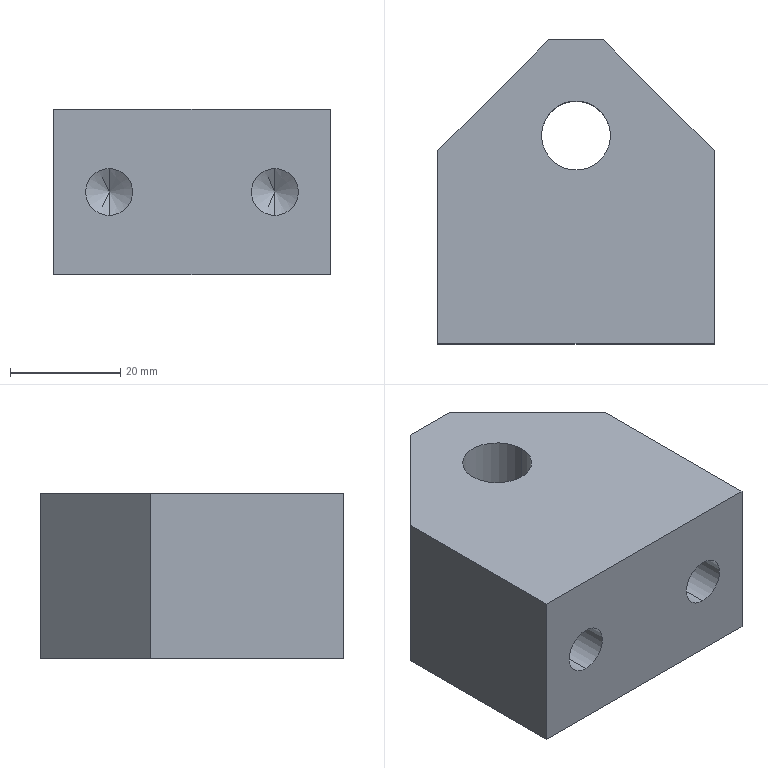Part | SolidWorks | features Chamfer 1, Extrusion 1, HoleWzd 1, ICE 1 | 1 solid | 18 faces | box 50 x 55 x 30 mm | volume 63941 mm3 | plane 8 | cylinder 6 | cone 4 | commonest cylinder face diameters 8.5 x4 12.5 x2
STEP:
#1=CARTESIAN_POINT('',(-6.25,10.2,0.));
#2=VERTEX_POINT('',#1);
#3=CARTESIAN_POINT('',(6.25,10.2,0.));
#4=VERTEX_POINT('',#3);
#5=CARTESIAN_POINT('',(0.,10.2,0.));
#6=DIRECTION('',(0.,0.,1.));
#7=DIRECTION('',(1.,0.,0.));
#8=AXIS2_PLACEMENT_3D('',#5,#6,#7);
#9=CIRCLE('',#8,6.25);
#10=EDGE_CURVE('',#2,#4,#9,.T.);
#11=ORIENTED_EDGE('',*,*,#10,.F.);
#12=CARTESIAN_POINT('',(-6.25,10.2,30.));
#13=VERTEX_POINT('',#12);
#14=CARTESIAN_POINT('',(-6.25,10.2,0.));
#15=DIRECTION('',(0.,0.,1.));
#16=VECTOR('',#15,1000.);
#17=LINE('',#14,#16);
#18=EDGE_CURVE('',#2,#13,#17,.T.);
#19=ORIENTED_EDGE('',*,*,#18,.T.);
#20=CARTESIAN_POINT('',(6.25,10.2,30.));
#21=VERTEX_POINT('',#20);
#22=CARTESIAN_POINT('',(0.,10.2,30.));
#23=DIRECTION('',(0.,0.,1.));
#24=DIRECTION('',(1.,0.,0.));
#25=AXIS2_PLACEMENT_3D('',#22,#23,#24);
#26=CIRCLE('',#25,6.25);
#27=EDGE_CURVE('',#13,#21,#26,.T.);
#28=ORIENTED_EDGE('',*,*,#27,.T.);
#29=CARTESIAN_POINT('',(6.25,10.2,0.));
#30=DIRECTION('',(0.,0.,1.));
#31=VECTOR('',#30,1000.);
#32=LINE('',#29,#31);
#33=EDGE_CURVE('',#4,#21,#32,.T.);
#34=ORIENTED_EDGE('',*,*,#33,.F.);
#35=EDGE_LOOP('',(#11,#19,#28,#34));
#36=FACE_OUTER_BOUND('',#35,.T.);
#37=CARTESIAN_POINT('',(0.,10.2,0.));
#38=DIRECTION('',(0.,0.,1.));
#39=DIRECTION('',(1.,0.,0.));
#40=AXIS2_PLACEMENT_3D('',#37,#38,#39);
#41=CYLINDRICAL_SURFACE('',#40,6.25);
#42=ADVANCED_FACE('',(#36),#41,.F.);
#43=CARTESIAN_POINT('',(-15.,-3.,19.25));
#44=VERTEX_POINT('',#43);
#45=CARTESIAN_POINT('',(-15.,-3.,10.75));
#46=VERTEX_POINT('',#45);
#47=CARTESIAN_POINT('',(-15.,-3.,15.));
#48=DIRECTION('',(0.,-1.,0.));
#49=DIRECTION('',(0.,0.,-1.));
#50=AXIS2_PLACEMENT_3D('',#47,#48,#49);
#51=CIRCLE('',#50,4.25);
#52=EDGE_CURVE('',#44,#46,#51,.T.);
#53=ORIENTED_EDGE('',*,*,#52,.F.);
#54=CARTESIAN_POINT('',(-15.,-27.5,19.25));
#55=VERTEX_POINT('',#54);
#56=CARTESIAN_POINT('',(-15.,-27.5,19.25));
#57=DIRECTION('',(0.,-1.,0.));
#58=VECTOR('',#57,1000.);
#59=LINE('',#56,#58);
#60=EDGE_CURVE('',#44,#55,#59,.T.);
#61=ORIENTED_EDGE('',*,*,#60,.T.);
#62=CARTESIAN_POINT('',(-15.,-27.5,10.75));
#63=VERTEX_POINT('',#62);
#64=CARTESIAN_POINT('',(-15.,-27.5,15.));
#65=DIRECTION('',(0.,-1.,0.));
#66=DIRECTION('',(0.,0.,-1.));
#67=AXIS2_PLACEMENT_3D('',#64,#65,#66);
#68=CIRCLE('',#67,4.25);
#69=EDGE_CURVE('',#55,#63,#68,.T.);
#70=ORIENTED_EDGE('',*,*,#69,.T.);
#71=CARTESIAN_POINT('',(-15.,-27.5,10.75));
#72=DIRECTION('',(0.,-1.,0.));
#73=VECTOR('',#72,1000.);
#74=LINE('',#71,#73);
#75=EDGE_CURVE('',#46,#63,#74,.T.);
#76=ORIENTED_EDGE('',*,*,#75,.F.);
#77=EDGE_LOOP('',(#53,#61,#70,#76));
#78=FACE_OUTER_BOUND('',#77,.T.);
#79=CARTESIAN_POINT('',(-15.,-27.5,15.));
#80=DIRECTION('',(0.,-1.,0.));
#81=DIRECTION('',(0.,0.,-1.));
#82=AXIS2_PLACEMENT_3D('',#79,#80,#81);
#83=CYLINDRICAL_SURFACE('',#82,4.25);
#84=ADVANCED_FACE('',(#78),#83,.F.);
#85=CARTESIAN_POINT('',(-15.,-0.4463,15.));
#86=VERTEX_POINT('',#85);
#87=CARTESIAN_POINT('',(-15.,-3.,10.75));
#88=DIRECTION('',(0.,-0.515,-0.8572));
#89=VECTOR('',#88,1000.);
#90=LINE('',#87,#89);
#91=EDGE_CURVE('',#86,#46,#90,.T.);
#92=ORIENTED_EDGE('',*,*,#91,.F.);
#93=CARTESIAN_POINT('',(-15.,-3.,19.25));
#94=DIRECTION('',(0.,-0.515,0.8572));
#95=VECTOR('',#94,1000.);
#96=LINE('',#93,#95);
#97=EDGE_CURVE('',#86,#44,#96,.T.);
#98=ORIENTED_EDGE('',*,*,#97,.T.);
#99=ORIENTED_EDGE('',*,*,#52,.T.);
#100=EDGE_LOOP('',(#92,#98,#99));
#101=FACE_OUTER_BOUND('',#100,.T.);
#102=CARTESIAN_POINT('',(-15.,-3.,15.));
#103=DIRECTION('',(0.,-1.,0.));
#104=DIRECTION('',(0.,0.,-1.));
#105=AXIS2_PLACEMENT_3D('',#102,#103,#104);
#106=CONICAL_SURFACE('',#105,4.25,1.03);
#107=ADVANCED_FACE('',(#101),#106,.F.);
#108=CARTESIAN_POINT('',(15.,-3.,19.25));
#109=VERTEX_POINT('',#108);
#110=CARTESIAN_POINT('',(15.,-3.,10.75));
#111=VERTEX_POINT('',#110);
#112=CARTESIAN_POINT('',(15.,-3.,15.));
#113=DIRECTION('',(0.,-1.,0.));
#114=DIRECTION('',(0.,0.,-1.));
#115=AXIS2_PLACEMENT_3D('',#112,#113,#114);
#116=CIRCLE('',#115,4.25);
#117=EDGE_CURVE('',#109,#111,#116,.T.);
#118=ORIENTED_EDGE('',*,*,#117,.F.);
#119=CARTESIAN_POINT('',(15.,-27.5,19.25));
#120=VERTEX_POINT('',#119);
#121=CARTESIAN_POINT('',(15.,-27.5,19.25));
#122=DIRECTION('',(0.,-1.,0.));
#123=VECTOR('',#122,1000.);
#124=LINE('',#121,#123);
#125=EDGE_CURVE('',#109,#120,#124,.T.);
#126=ORIENTED_EDGE('',*,*,#125,.T.);
#127=CARTESIAN_POINT('',(15.,-27.5,10.75));
#128=VERTEX_POINT('',#127);
#129=CARTESIAN_POINT('',(15.,-27.5,15.));
#130=DIRECTION('',(0.,-1.,0.));
#131=DIRECTION('',(0.,0.,-1.));
#132=AXIS2_PLACEMENT_3D('',#129,#130,#131);
#133=CIRCLE('',#132,4.25);
#134=EDGE_CURVE('',#120,#128,#133,.T.);
#135=ORIENTED_EDGE('',*,*,#134,.T.);
#136=CARTESIAN_POINT('',(15.,-27.5,10.75));
#137=DIRECTION('',(0.,-1.,0.));
#138=VECTOR('',#137,1000.);
#139=LINE('',#136,#138);
#140=EDGE_CURVE('',#111,#128,#139,.T.);
#141=ORIENTED_EDGE('',*,*,#140,.F.);
#142=EDGE_LOOP('',(#118,#126,#135,#141));
#143=FACE_OUTER_BOUND('',#142,.T.);
#144=CARTESIAN_POINT('',(15.,-27.5,15.));
#145=DIRECTION('',(0.,-1.,0.));
#146=DIRECTION('',(0.,0.,-1.));
#147=AXIS2_PLACEMENT_3D('',#144,#145,#146);
#148=CYLINDRICAL_SURFACE('',#147,4.25);
#149=ADVANCED_FACE('',(#143),#148,.F.);
#150=CARTESIAN_POINT('',(15.,-0.4463,15.));
#151=VERTEX_POINT('',#150);
#152=CARTESIAN_POINT('',(15.,-3.,10.75));
#153=DIRECTION('',(0.,-0.515,-0.8572));
#154=VECTOR('',#153,1000.);
#155=LINE('',#152,#154);
#156=EDGE_CURVE('',#151,#111,#155,.T.);
#157=ORIENTED_EDGE('',*,*,#156,.F.);
#158=CARTESIAN_POINT('',(15.,-3.,19.25));
#159=DIRECTION('',(0.,-0.515,0.8572));
#160=VECTOR('',#159,1000.);
#161=LINE('',#158,#160);
#162=EDGE_CURVE('',#151,#109,#161,.T.);
#163=ORIENTED_EDGE('',*,*,#162,.T.);
#164=ORIENTED_EDGE('',*,*,#117,.T.);
#165=EDGE_LOOP('',(#157,#163,#164));
#166=FACE_OUTER_BOUND('',#165,.T.);
#167=CARTESIAN_POINT('',(15.,-3.,15.));
#168=DIRECTION('',(0.,-1.,0.));
#169=DIRECTION('',(0.,0.,-1.));
#170=AXIS2_PLACEMENT_3D('',#167,#168,#169);
#171=CONICAL_SURFACE('',#170,4.25,1.03);
#172=ADVANCED_FACE('',(#166),#171,.F.);
#173=CARTESIAN_POINT('',(25.,-27.5,0.));
#174=VERTEX_POINT('',#173);
#175=CARTESIAN_POINT('',(25.,7.5,0.));
#176=VERTEX_POINT('',#175);
#177=CARTESIAN_POINT('',(25.,27.5,0.));
#178=DIRECTION('',(0.,1.,0.));
#179=VECTOR('',#178,1000.);
#180=LINE('',#177,#179);
#181=EDGE_CURVE('',#174,#176,#180,.T.);
#182=ORIENTED_EDGE('',*,*,#181,.T.);
#183=CARTESIAN_POINT('',(25.,7.5,30.));
#184=VERTEX_POINT('',#183);
#185=CARTESIAN_POINT('',(25.,7.5,30.));
#186=DIRECTION('',(0.,0.,1.));
#187=VECTOR('',#186,1000.);
#188=LINE('',#185,#187);
#189=EDGE_CURVE('',#176,#184,#188,.T.);
#190=ORIENTED_EDGE('',*,*,#189,.T.);
#191=CARTESIAN_POINT('',(25.,-27.5,30.));
#192=VERTEX_POINT('',#191);
#193=CARTESIAN_POINT('',(25.,27.5,30.));
#194=DIRECTION('',(0.,1.,0.));
#195=VECTOR('',#194,1000.);
#196=LINE('',#193,#195);
#197=EDGE_CURVE('',#192,#184,#196,.T.);
#198=ORIENTED_EDGE('',*,*,#197,.F.);
#199=CARTESIAN_POINT('',(25.,-27.5,30.));
#200=DIRECTION('',(0.,0.,-1.));
#201=VECTOR('',#200,1000.);
#202=LINE('',#199,#201);
#203=EDGE_CURVE('',#192,#174,#202,.T.);
#204=ORIENTED_EDGE('',*,*,#203,.T.);
#205=EDGE_LOOP('',(#182,#190,#198,#204));
#206=FACE_OUTER_BOUND('',#205,.T.);
#207=CARTESIAN_POINT('',(25.,27.5,30.));
#208=DIRECTION('',(-1.,0.,0.));
#209=DIRECTION('',(0.,-1.,0.));
#210=AXIS2_PLACEMENT_3D('',#207,#208,#209);
#211=PLANE('',#210);
#212=ADVANCED_FACE('',(#206),#211,.F.);
#213=CARTESIAN_POINT('',(5.,27.5,30.));
#214=VERTEX_POINT('',#213);
#215=CARTESIAN_POINT('',(-5.,27.5,30.));
#216=VERTEX_POINT('',#215);
#217=CARTESIAN_POINT('',(-25.,27.5,30.));
#218=DIRECTION('',(-1.,0.,0.));
#219=VECTOR('',#218,1000.);
#220=LINE('',#217,#219);
#221=EDGE_CURVE('',#214,#216,#220,.T.);
#222=ORIENTED_EDGE('',*,*,#221,.F.);
#223=CARTESIAN_POINT('',(5.,27.5,0.));
#224=VERTEX_POINT('',#223);
#225=CARTESIAN_POINT('',(5.,27.5,30.));
#226=DIRECTION('',(0.,0.,-1.));
#227=VECTOR('',#226,1000.);
#228=LINE('',#225,#227);
#229=EDGE_CURVE('',#214,#224,#228,.T.);
#230=ORIENTED_EDGE('',*,*,#229,.T.);
#231=CARTESIAN_POINT('',(-5.,27.5,0.));
#232=VERTEX_POINT('',#231);
#233=CARTESIAN_POINT('',(-25.,27.5,0.));
#234=DIRECTION('',(-1.,0.,0.));
#235=VECTOR('',#234,1000.);
#236=LINE('',#233,#235);
#237=EDGE_CURVE('',#224,#232,#236,.T.);
#238=ORIENTED_EDGE('',*,*,#237,.T.);
#239=CARTESIAN_POINT('',(-5.,27.5,30.));
#240=DIRECTION('',(0.,0.,1.));
#241=VECTOR('',#240,1000.);
#242=LINE('',#239,#241);
#243=EDGE_CURVE('',#232,#216,#242,.T.);
#244=ORIENTED_EDGE('',*,*,#243,.T.);
#245=EDGE_LOOP('',(#222,#230,#238,#244));
#246=FACE_OUTER_BOUND('',#245,.T.);
#247=CARTESIAN_POINT('',(-25.,27.5,30.));
#248=DIRECTION('',(0.,-1.,0.));
#249=DIRECTION('',(0.,0.,-1.));
#250=AXIS2_PLACEMENT_3D('',#247,#248,#249);
#251=PLANE('',#250);
#252=ADVANCED_FACE('',(#246),#251,.F.);
#253=CARTESIAN_POINT('',(-25.,7.5,30.));
#254=VERTEX_POINT('',#253);
#255=CARTESIAN_POINT('',(-25.,-27.5,30.));
#256=VERTEX_POINT('',#255);
#257=CARTESIAN_POINT('',(-25.,27.5,30.));
#258=DIRECTION('',(0.,-1.,0.));
#259=VECTOR('',#258,1000.);
#260=LINE('',#257,#259);
#261=EDGE_CURVE('',#254,#256,#260,.T.);
#262=ORIENTED_EDGE('',*,*,#261,.F.);
#263=CARTESIAN_POINT('',(-25.,7.5,0.));
#264=VERTEX_POINT('',#263);
#265=CARTESIAN_POINT('',(-25.,7.5,30.));
#266=DIRECTION('',(0.,0.,-1.));
#267=VECTOR('',#266,1000.);
#268=LINE('',#265,#267);
#269=EDGE_CURVE('',#254,#264,#268,.T.);
#270=ORIENTED_EDGE('',*,*,#269,.T.);
#271=CARTESIAN_POINT('',(-25.,-27.5,0.));
#272=VERTEX_POINT('',#271);
#273=CARTESIAN_POINT('',(-25.,27.5,0.));
#274=DIRECTION('',(0.,-1.,0.));
#275=VECTOR('',#274,1000.);
#276=LINE('',#273,#275);
#277=EDGE_CURVE('',#264,#272,#276,.T.);
#278=ORIENTED_EDGE('',*,*,#277,.T.);
#279=CARTESIAN_POINT('',(-25.,-27.5,30.));
#280=DIRECTION('',(0.,0.,-1.));
#281=VECTOR('',#280,1000.);
#282=LINE('',#279,#281);
#283=EDGE_CURVE('',#256,#272,#282,.T.);
#284=ORIENTED_EDGE('',*,*,#283,.F.);
#285=EDGE_LOOP('',(#262,#270,#278,#284));
#286=FACE_OUTER_BOUND('',#285,.T.);
#287=CARTESIAN_POINT('',(-25.,27.5,30.));
#288=DIRECTION('',(1.,0.,0.));
#289=DIRECTION('',(0.,1.,0.));
#290=AXIS2_PLACEMENT_3D('',#287,#288,#289);
#291=PLANE('',#290);
#292=ADVANCED_FACE('',(#286),#291,.F.);
#293=CARTESIAN_POINT('',(-15.,-27.5,15.));
#294=DIRECTION('',(0.,-1.,0.));
#295=DIRECTION('',(0.,0.,-1.));
#296=AXIS2_PLACEMENT_3D('',#293,#294,#295);
#297=CIRCLE('',#296,4.25);
#298=EDGE_CURVE('',#63,#55,#297,.T.);
#299=ORIENTED_EDGE('',*,*,#298,.F.);
#300=ORIENTED_EDGE('',*,*,#69,.F.);
#301=EDGE_LOOP('',(#299,#300));
#302=FACE_BOUND('',#301,.T.);
#303=CARTESIAN_POINT('',(15.,-27.5,15.));
#304=DIRECTION('',(0.,-1.,0.));
#305=DIRECTION('',(0.,0.,-1.));
#306=AXIS2_PLACEMENT_3D('',#303,#304,#305);
#307=CIRCLE('',#306,4.25);
#308=EDGE_CURVE('',#128,#120,#307,.T.);
#309=ORIENTED_EDGE('',*,*,#308,.F.);
#310=ORIENTED_EDGE('',*,*,#134,.F.);
#311=EDGE_LOOP('',(#309,#310));
#312=FACE_BOUND('',#311,.T.);
#313=CARTESIAN_POINT('',(-25.,-27.5,0.));
#314=DIRECTION('',(1.,0.,0.));
#315=VECTOR('',#314,1000.);
#316=LINE('',#313,#315);
#317=EDGE_CURVE('',#272,#174,#316,.T.);
#318=ORIENTED_EDGE('',*,*,#317,.T.);
#319=ORIENTED_EDGE('',*,*,#203,.F.);
#320=CARTESIAN_POINT('',(-25.,-27.5,30.));
#321=DIRECTION('',(1.,0.,0.));
#322=VECTOR('',#321,1000.);
#323=LINE('',#320,#322);
#324=EDGE_CURVE('',#256,#192,#323,.T.);
#325=ORIENTED_EDGE('',*,*,#324,.F.);
#326=ORIENTED_EDGE('',*,*,#283,.T.);
#327=EDGE_LOOP('',(#318,#319,#325,#326));
#328=FACE_OUTER_BOUND('',#327,.T.);
#329=CARTESIAN_POINT('',(-25.,-27.5,30.));
#330=DIRECTION('',(0.,1.,0.));
#331=DIRECTION('',(0.,0.,1.));
#332=AXIS2_PLACEMENT_3D('',#329,#330,#331);
#333=PLANE('',#332);
#334=ADVANCED_FACE('',(#302,#312,#328),#333,.F.);
#335=CARTESIAN_POINT('',(0.,10.2,30.));
#336=DIRECTION('',(0.,0.,1.));
#337=DIRECTION('',(1.,0.,0.));
#338=AXIS2_PLACEMENT_3D('',#335,#336,#337);
#339=CIRCLE('',#338,6.25);
#340=EDGE_CURVE('',#21,#13,#339,.T.);
#341=ORIENTED_EDGE('',*,*,#340,.F.);
#342=ORIENTED_EDGE('',*,*,#27,.F.);
#343=EDGE_LOOP('',(#341,#342));
#344=FACE_BOUND('',#343,.T.);
#345=ORIENTED_EDGE('',*,*,#197,.T.);
#346=CARTESIAN_POINT('',(16.25,16.25,30.));
#347=DIRECTION('',(-0.7071,0.7071,0.));
#348=VECTOR('',#347,1000.);
#349=LINE('',#346,#348);
#350=EDGE_CURVE('',#184,#214,#349,.T.);
#351=ORIENTED_EDGE('',*,*,#350,.T.);
#352=ORIENTED_EDGE('',*,*,#221,.T.);
#353=CARTESIAN_POINT('',(-16.25,16.25,30.));
#354=DIRECTION('',(-0.7071,-0.7071,0.));
#355=VECTOR('',#354,1000.);
#356=LINE('',#353,#355);
#357=EDGE_CURVE('',#216,#254,#356,.T.);
#358=ORIENTED_EDGE('',*,*,#357,.T.);
#359=ORIENTED_EDGE('',*,*,#261,.T.);
#360=ORIENTED_EDGE('',*,*,#324,.T.);
#361=EDGE_LOOP('',(#345,#351,#352,#358,#359,#360));
#362=FACE_OUTER_BOUND('',#361,.T.);
#363=CARTESIAN_POINT('',(0.,0.,30.));
#364=DIRECTION('',(0.,0.,1.));
#365=DIRECTION('',(1.,0.,0.));
#366=AXIS2_PLACEMENT_3D('',#363,#364,#365);
#367=PLANE('',#366);
#368=ADVANCED_FACE('',(#344,#362),#367,.T.);
#369=CARTESIAN_POINT('',(0.,10.2,0.));
#370=DIRECTION('',(0.,0.,1.));
#371=DIRECTION('',(1.,0.,0.));
#372=AXIS2_PLACEMENT_3D('',#369,#370,#371);
#373=CIRCLE('',#372,6.25);
#374=EDGE_CURVE('',#4,#2,#373,.T.);
#375=ORIENTED_EDGE('',*,*,#374,.T.);
#376=ORIENTED_EDGE('',*,*,#10,.T.);
#377=EDGE_LOOP('',(#375,#376));
#378=FACE_BOUND('',#377,.T.);
#379=ORIENTED_EDGE('',*,*,#237,.F.);
#380=CARTESIAN_POINT('',(5.,27.5,0.));
#381=DIRECTION('',(0.7071,-0.7071,0.));
#382=VECTOR('',#381,1000.);
#383=LINE('',#380,#382);
#384=EDGE_CURVE('',#224,#176,#383,.T.);
#385=ORIENTED_EDGE('',*,*,#384,.T.);
#386=ORIENTED_EDGE('',*,*,#181,.F.);
#387=ORIENTED_EDGE('',*,*,#317,.F.);
#388=ORIENTED_EDGE('',*,*,#277,.F.);
#389=CARTESIAN_POINT('',(-25.,7.5,0.));
#390=DIRECTION('',(0.7071,0.7071,0.));
#391=VECTOR('',#390,1000.);
#392=LINE('',#389,#391);
#393=EDGE_CURVE('',#264,#232,#392,.T.);
#394=ORIENTED_EDGE('',*,*,#393,.T.);
#395=EDGE_LOOP('',(#379,#385,#386,#387,#388,#394));
#396=FACE_OUTER_BOUND('',#395,.T.);
#397=CARTESIAN_POINT('',(0.,0.,0.));
#398=DIRECTION('',(0.,0.,1.));
#399=DIRECTION('',(1.,0.,0.));
#400=AXIS2_PLACEMENT_3D('',#397,#398,#399);
#401=PLANE('',#400);
#402=ADVANCED_FACE('',(#378,#396),#401,.F.);
#403=ORIENTED_EDGE('',*,*,#350,.F.);
#404=ORIENTED_EDGE('',*,*,#189,.F.);
#405=ORIENTED_EDGE('',*,*,#384,.F.);
#406=ORIENTED_EDGE('',*,*,#229,.F.);
#407=EDGE_LOOP('',(#403,#404,#405,#406));
#408=FACE_OUTER_BOUND('',#407,.T.);
#409=CARTESIAN_POINT('',(5.,27.5,30.));
#410=DIRECTION('',(-0.7071,-0.7071,0.));
#411=DIRECTION('',(0.,0.,-1.));
#412=AXIS2_PLACEMENT_3D('',#409,#410,#411);
#413=PLANE('',#412);
#414=ADVANCED_FACE('',(#408),#413,.F.);
#415=ORIENTED_EDGE('',*,*,#357,.F.);
#416=ORIENTED_EDGE('',*,*,#243,.F.);
#417=ORIENTED_EDGE('',*,*,#393,.F.);
#418=ORIENTED_EDGE('',*,*,#269,.F.);
#419=EDGE_LOOP('',(#415,#416,#417,#418));
#420=FACE_OUTER_BOUND('',#419,.T.);
#421=CARTESIAN_POINT('',(-25.,7.5,30.));
#422=DIRECTION('',(0.7071,-0.7071,0.));
#423=DIRECTION('',(0.,0.,-1.));
#424=AXIS2_PLACEMENT_3D('',#421,#422,#423);
#425=PLANE('',#424);
#426=ADVANCED_FACE('',(#420),#425,.F.);
#427=ORIENTED_EDGE('',*,*,#162,.F.);
#428=ORIENTED_EDGE('',*,*,#156,.T.);
#429=CARTESIAN_POINT('',(15.,-3.,15.));
#430=DIRECTION('',(0.,-1.,0.));
#431=DIRECTION('',(0.,0.,-1.));
#432=AXIS2_PLACEMENT_3D('',#429,#430,#431);
#433=CIRCLE('',#432,4.25);
#434=EDGE_CURVE('',#111,#109,#433,.T.);
#435=ORIENTED_EDGE('',*,*,#434,.T.);
#436=EDGE_LOOP('',(#427,#428,#435));
#437=FACE_OUTER_BOUND('',#436,.T.);
#438=CARTESIAN_POINT('',(15.,-3.,15.));
#439=DIRECTION('',(0.,-1.,0.));
#440=DIRECTION('',(0.,0.,-1.));
#441=AXIS2_PLACEMENT_3D('',#438,#439,#440);
#442=CONICAL_SURFACE('',#441,4.25,1.03);
#443=ADVANCED_FACE('',(#437),#442,.F.);
#444=ORIENTED_EDGE('',*,*,#125,.F.);
#445=ORIENTED_EDGE('',*,*,#434,.F.);
#446=ORIENTED_EDGE('',*,*,#140,.T.);
#447=ORIENTED_EDGE('',*,*,#308,.T.);
#448=EDGE_LOOP('',(#444,#445,#446,#447));
#449=FACE_OUTER_BOUND('',#448,.T.);
#450=CARTESIAN_POINT('',(15.,-27.5,15.));
#451=DIRECTION('',(0.,-1.,0.));
#452=DIRECTION('',(0.,0.,-1.));
#453=AXIS2_PLACEMENT_3D('',#450,#451,#452);
#454=CYLINDRICAL_SURFACE('',#453,4.25);
#455=ADVANCED_FACE('',(#449),#454,.F.);
#456=ORIENTED_EDGE('',*,*,#97,.F.);
#457=ORIENTED_EDGE('',*,*,#91,.T.);
#458=CARTESIAN_POINT('',(-15.,-3.,15.));
#459=DIRECTION('',(0.,-1.,0.));
#460=DIRECTION('',(0.,0.,-1.));
#461=AXIS2_PLACEMENT_3D('',#458,#459,#460);
#462=CIRCLE('',#461,4.25);
#463=EDGE_CURVE('',#46,#44,#462,.T.);
#464=ORIENTED_EDGE('',*,*,#463,.T.);
#465=EDGE_LOOP('',(#456,#457,#464));
#466=FACE_OUTER_BOUND('',#465,.T.);
#467=CARTESIAN_POINT('',(-15.,-3.,15.));
#468=DIRECTION('',(0.,-1.,0.));
#469=DIRECTION('',(0.,0.,-1.));
#470=AXIS2_PLACEMENT_3D('',#467,#468,#469);
#471=CONICAL_SURFACE('',#470,4.25,1.03);
#472=ADVANCED_FACE('',(#466),#471,.F.);
#473=ORIENTED_EDGE('',*,*,#60,.F.);
#474=ORIENTED_EDGE('',*,*,#463,.F.);
#475=ORIENTED_EDGE('',*,*,#75,.T.);
#476=ORIENTED_EDGE('',*,*,#298,.T.);
#477=EDGE_LOOP('',(#473,#474,#475,#476));
#478=FACE_OUTER_BOUND('',#477,.T.);
#479=CARTESIAN_POINT('',(-15.,-27.5,15.));
#480=DIRECTION('',(0.,-1.,0.));
#481=DIRECTION('',(0.,0.,-1.));
#482=AXIS2_PLACEMENT_3D('',#479,#480,#481);
#483=CYLINDRICAL_SURFACE('',#482,4.25);
#484=ADVANCED_FACE('',(#478),#483,.F.);
#485=ORIENTED_EDGE('',*,*,#18,.F.);
#486=ORIENTED_EDGE('',*,*,#374,.F.);
#487=ORIENTED_EDGE('',*,*,#33,.T.);
#488=ORIENTED_EDGE('',*,*,#340,.T.);
#489=EDGE_LOOP('',(#485,#486,#487,#488));
#490=FACE_OUTER_BOUND('',#489,.T.);
#491=CARTESIAN_POINT('',(0.,10.2,0.));
#492=DIRECTION('',(0.,0.,1.));
#493=DIRECTION('',(1.,0.,0.));
#494=AXIS2_PLACEMENT_3D('',#491,#492,#493);
#495=CYLINDRICAL_SURFACE('',#494,6.25);
#496=ADVANCED_FACE('',(#490),#495,.F.);
#497=CLOSED_SHELL('',(#42,#84,#107,#149,#172,#212,#252,#292,#334,#368,#402,#414,#426,#443,#455,#472,#484,#496));
#498=MANIFOLD_SOLID_BREP('',#497);
#499=CARTESIAN_POINT('',(0.,0.,0.));
#500=DIRECTION('',(0.,0.,1.));
#501=DIRECTION('',(1.,0.,0.));
#502=AXIS2_PLACEMENT_3D('',#499,#500,#501);
#503=(LENGTH_UNIT()NAMED_UNIT(*)SI_UNIT(.MILLI.,.METRE.));
#504=UNCERTAINTY_MEASURE_WITH_UNIT(LENGTH_MEASURE(0.00001),#503,'','');
#505=(NAMED_UNIT(*)PLANE_ANGLE_UNIT()SI_UNIT($,.RADIAN.));
#506=(NAMED_UNIT(*)SI_UNIT($,.STERADIAN.)SOLID_ANGLE_UNIT());
#507=(GEOMETRIC_REPRESENTATION_CONTEXT(3)GLOBAL_UNCERTAINTY_ASSIGNED_CONTEXT((#504))GLOBAL_UNIT_ASSIGNED_CONTEXT((#503,#505,#506))REPRESENTATION_CONTEXT('',''));
#508=ADVANCED_BREP_SHAPE_REPRESENTATION('',(#498,#502),#507);